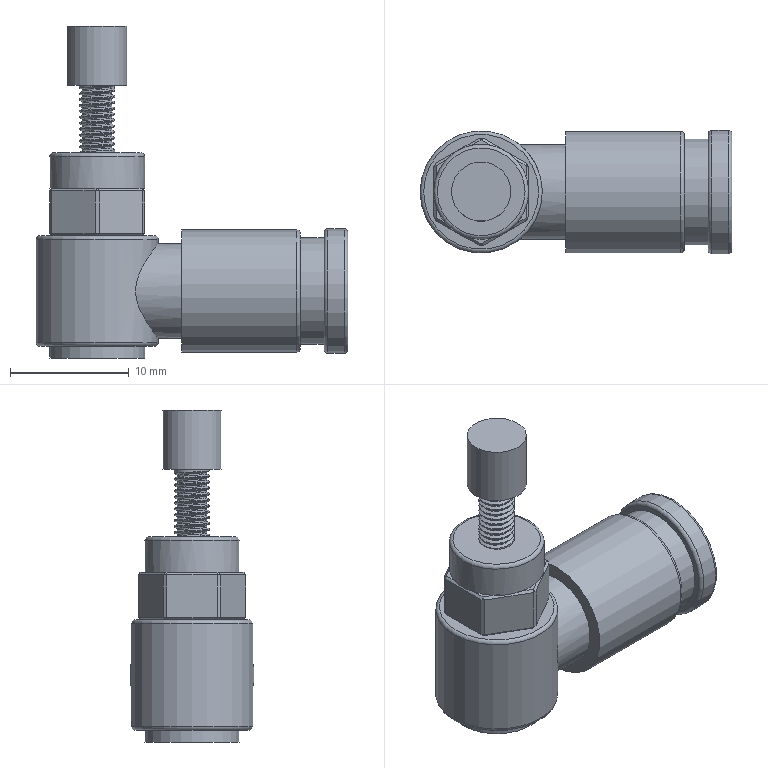Part | STEP file | Tube feed_id10_x_t | 1 solid | 82 faces | box 26.3 x 10.5 x 28 mm | volume 2522 mm3 | plane 61 | cylinder 11 | torus 6 | spline 4 | commonest cylinder face diameters 8 x3 10.3 x2 2.5 x1 3 x1 5 x1 6 x1